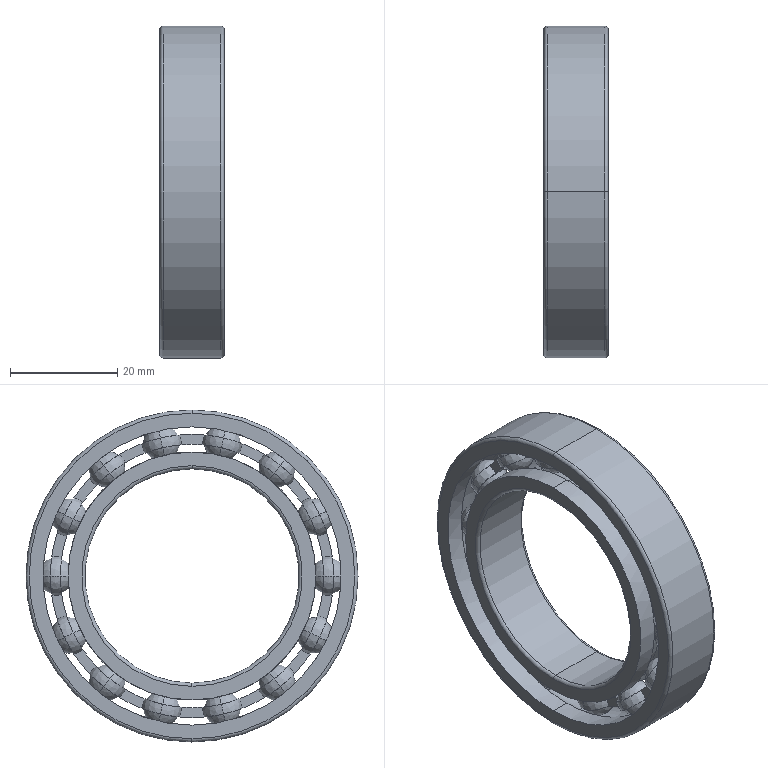Part | SolidWorks | 1 solid | 213 faces | box 12 x 62 x 62 mm | volume 13593 mm3 | sphere 112 | torus 53 | plane 32 | cylinder 16 | commonest cylinder face diameters 46.3 x4 55.7 x4 40 x2 49.145 x2 52.855 x2 62 x2